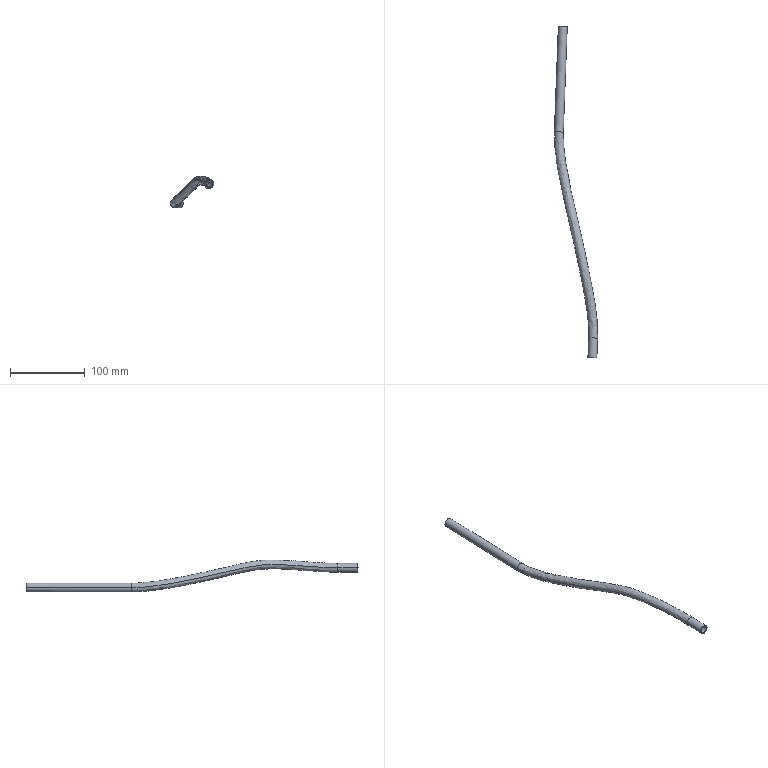Part | SolidWorks | features 3DProfileFeature 2, Sweep 1 | 1 solid | 14 faces | box 58.081 x 444.507 x 42.863 mm | volume 15608 mm3 | cylinder 8 | spline 4 | plane 2 | commonest cylinder face diameters 10 x4 12 x4